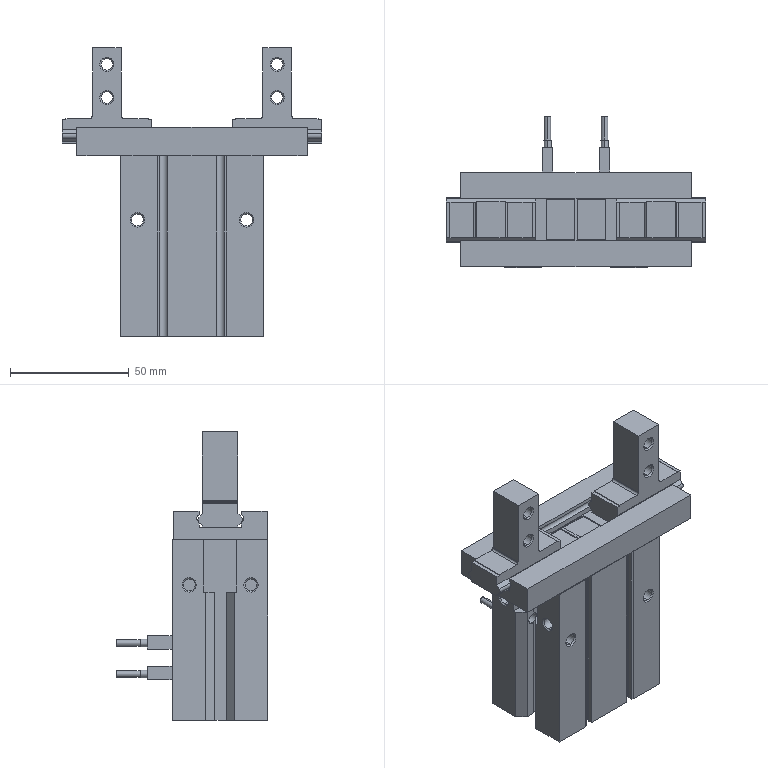Part | SolidWorks | features AEMSimFeature 1, MirrorCompFeat 1, ReferencePattern 1 | 5 solids | 313 faces | box 109.088 x 63.7 x 121.5 mm | volume 211309 mm3 | plane 191 | cylinder 80 | cone 42 | commonest cylinder face diameters 4.917 x24 4 x14 5.1 x8 2.1 x6 1.6 x4 2.5 x4